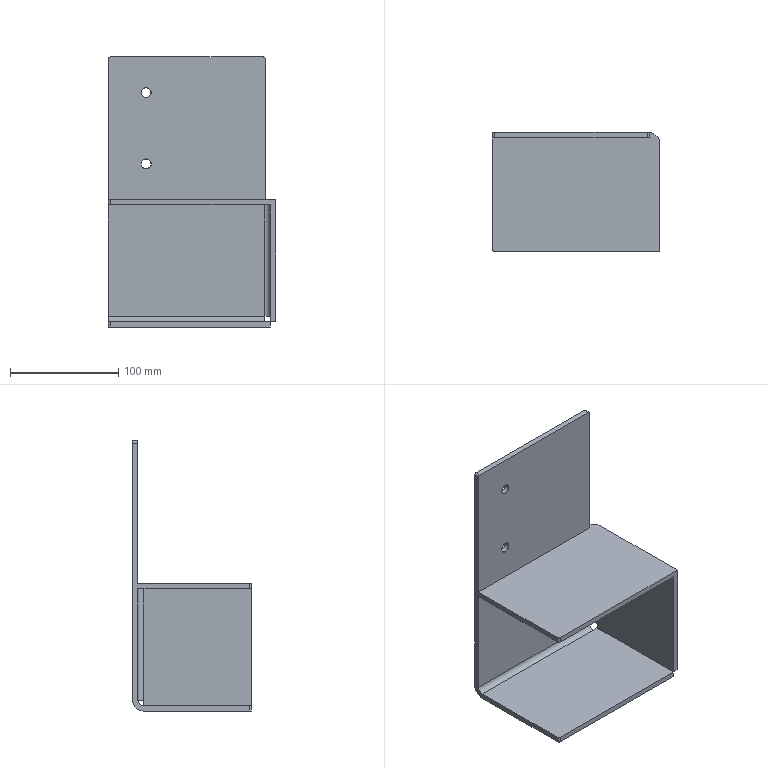Part | NX | 1 solid | 36 faces | box 155 x 110 x 250 mm | volume 398731 mm3 | plane 20 | cylinder 12 | cone 4 | commonest cylinder face diameters 4 x4 9 x4 10 x2 20 x2
STEP:
#1=CARTESIAN_POINT('',(44.,-222.5,-167.429));
#2=VERTEX_POINT('',#1);
#3=CARTESIAN_POINT('',(49.,-222.5,-167.429));
#4=VERTEX_POINT('',#3);
#5=CARTESIAN_POINT('',(49.,-222.5,-167.429));
#6=DIRECTION('',(1.,0.,0.));
#7=VECTOR('',#6,1000.);
#8=LINE('',#5,#7);
#9=EDGE_CURVE('',#2,#4,#8,.T.);
#10=ORIENTED_EDGE('',*,*,#9,.T.);
#11=CARTESIAN_POINT('',(49.,-322.5,-167.429));
#12=VERTEX_POINT('',#11);
#13=CARTESIAN_POINT('',(49.,-212.5,-167.429));
#14=DIRECTION('',(0.,-1.,0.));
#15=VECTOR('',#14,1000.);
#16=LINE('',#13,#15);
#17=EDGE_CURVE('',#4,#12,#16,.T.);
#18=ORIENTED_EDGE('',*,*,#17,.T.);
#19=CARTESIAN_POINT('',(44.,-322.5,-167.429));
#20=VERTEX_POINT('',#19);
#21=CARTESIAN_POINT('',(-35.923,-322.5,-167.429));
#22=DIRECTION('',(-1.,0.,0.));
#23=VECTOR('',#22,1000.);
#24=LINE('',#21,#23);
#25=EDGE_CURVE('',#12,#20,#24,.T.);
#26=ORIENTED_EDGE('',*,*,#25,.T.);
#27=CARTESIAN_POINT('',(44.,-212.5,-167.429));
#28=DIRECTION('',(0.,1.,0.));
#29=VECTOR('',#28,1000.);
#30=LINE('',#27,#29);
#31=EDGE_CURVE('',#20,#2,#30,.T.);
#32=ORIENTED_EDGE('',*,*,#31,.T.);
#33=EDGE_LOOP('',(#10,#18,#26,#32));
#34=FACE_BOUND('',#33,.T.);
#35=CARTESIAN_POINT('',(44.,-247.5,-167.429));
#36=DIRECTION('',(0.,0.,-1.));
#37=DIRECTION('',(0.,-1.,0.));
#38=AXIS2_PLACEMENT_3D('',#35,#36,#37);
#39=PLANE('',#38);
#40=ADVANCED_FACE('',(#34),#39,.T.);
#41=CARTESIAN_POINT('',(-106.,-320.5,-172.5));
#42=VERTEX_POINT('',#41);
#43=CARTESIAN_POINT('',(-106.,-320.5,-167.5));
#44=VERTEX_POINT('',#43);
#45=CARTESIAN_POINT('',(-106.,-320.5,-67.481));
#46=DIRECTION('',(0.,0.,1.));
#47=VECTOR('',#46,1000.);
#48=LINE('',#45,#47);
#49=EDGE_CURVE('',#42,#44,#48,.T.);
#50=ORIENTED_EDGE('',*,*,#49,.T.);
#51=CARTESIAN_POINT('',(-106.,-222.5,-167.5));
#52=VERTEX_POINT('',#51);
#53=CARTESIAN_POINT('',(-106.,-212.5,-167.5));
#54=DIRECTION('',(0.,1.,0.));
#55=VECTOR('',#54,1000.);
#56=LINE('',#53,#55);
#57=EDGE_CURVE('',#44,#52,#56,.T.);
#58=ORIENTED_EDGE('',*,*,#57,.T.);
#59=CARTESIAN_POINT('',(-106.,-217.5,-162.5));
#60=VERTEX_POINT('',#59);
#61=CARTESIAN_POINT('',(-106.,-222.5,-162.5));
#62=DIRECTION('',(1.,0.,0.));
#63=DIRECTION('',(0.,0.,-1.));
#64=AXIS2_PLACEMENT_3D('',#61,#62,#63);
#65=CIRCLE('',#64,5.);
#66=EDGE_CURVE('',#52,#60,#65,.T.);
#67=ORIENTED_EDGE('',*,*,#66,.T.);
#68=CARTESIAN_POINT('',(-106.,-217.5,-59.5));
#69=VERTEX_POINT('',#68);
#70=CARTESIAN_POINT('',(-106.,-217.5,-67.481));
#71=DIRECTION('',(0.,0.,1.));
#72=VECTOR('',#71,1000.);
#73=LINE('',#70,#72);
#74=EDGE_CURVE('',#60,#69,#73,.T.);
#75=ORIENTED_EDGE('',*,*,#74,.T.);
#76=CARTESIAN_POINT('',(-106.,-320.5,-59.5));
#77=VERTEX_POINT('',#76);
#78=CARTESIAN_POINT('',(-106.,-212.5,-59.5));
#79=DIRECTION('',(0.,-1.,0.));
#80=VECTOR('',#79,1000.);
#81=LINE('',#78,#80);
#82=EDGE_CURVE('',#69,#77,#81,.T.);
#83=ORIENTED_EDGE('',*,*,#82,.T.);
#84=CARTESIAN_POINT('',(-106.,-320.5,-54.5));
#85=VERTEX_POINT('',#84);
#86=CARTESIAN_POINT('',(-106.,-320.5,-67.481));
#87=DIRECTION('',(0.,0.,1.));
#88=VECTOR('',#87,1000.);
#89=LINE('',#86,#88);
#90=EDGE_CURVE('',#77,#85,#89,.T.);
#91=ORIENTED_EDGE('',*,*,#90,.T.);
#92=CARTESIAN_POINT('',(-106.,-217.5,-54.5));
#93=VERTEX_POINT('',#92);
#94=CARTESIAN_POINT('',(-106.,-212.5,-54.5));
#95=DIRECTION('',(0.,1.,0.));
#96=VECTOR('',#95,1000.);
#97=LINE('',#94,#96);
#98=EDGE_CURVE('',#85,#93,#97,.T.);
#99=ORIENTED_EDGE('',*,*,#98,.T.);
#100=CARTESIAN_POINT('',(-106.,-217.5,75.5));
#101=VERTEX_POINT('',#100);
#102=CARTESIAN_POINT('',(-106.,-217.5,-67.481));
#103=DIRECTION('',(0.,0.,1.));
#104=VECTOR('',#103,1000.);
#105=LINE('',#102,#104);
#106=EDGE_CURVE('',#93,#101,#105,.T.);
#107=ORIENTED_EDGE('',*,*,#106,.T.);
#108=CARTESIAN_POINT('',(-106.,-212.5,75.5));
#109=VERTEX_POINT('',#108);
#110=CARTESIAN_POINT('',(-106.,-212.5,75.5));
#111=DIRECTION('',(0.,-1.,0.));
#112=VECTOR('',#111,1000.);
#113=LINE('',#110,#112);
#114=EDGE_CURVE('',#109,#101,#113,.T.);
#115=ORIENTED_EDGE('',*,*,#114,.F.);
#116=CARTESIAN_POINT('',(-106.,-212.5,-162.5));
#117=VERTEX_POINT('',#116);
#118=CARTESIAN_POINT('',(-106.,-212.5,-67.481));
#119=DIRECTION('',(0.,0.,-1.));
#120=VECTOR('',#119,1000.);
#121=LINE('',#118,#120);
#122=EDGE_CURVE('',#109,#117,#121,.T.);
#123=ORIENTED_EDGE('',*,*,#122,.T.);
#124=CARTESIAN_POINT('',(-106.,-222.5,-172.5));
#125=VERTEX_POINT('',#124);
#126=CARTESIAN_POINT('',(-106.,-222.5,-162.5));
#127=DIRECTION('',(1.,0.,0.));
#128=DIRECTION('',(0.,0.,-1.));
#129=AXIS2_PLACEMENT_3D('',#126,#127,#128);
#130=CIRCLE('',#129,10.);
#131=EDGE_CURVE('',#125,#117,#130,.T.);
#132=ORIENTED_EDGE('',*,*,#131,.F.);
#133=CARTESIAN_POINT('',(-106.,-212.5,-172.5));
#134=DIRECTION('',(0.,-1.,0.));
#135=VECTOR('',#134,1000.);
#136=LINE('',#133,#135);
#137=EDGE_CURVE('',#125,#42,#136,.T.);
#138=ORIENTED_EDGE('',*,*,#137,.T.);
#139=EDGE_LOOP('',(#50,#58,#67,#75,#83,#91,#99,#107,#115,#123,#132,#138));
#140=FACE_BOUND('',#139,.T.);
#141=CARTESIAN_POINT('',(-106.,-212.5,-85.5));
#142=DIRECTION('',(-1.,0.,0.));
#143=DIRECTION('',(0.,0.,1.));
#144=AXIS2_PLACEMENT_3D('',#141,#142,#143);
#145=PLANE('',#144);
#146=ADVANCED_FACE('',(#140),#145,.T.);
#147=ORIENTED_EDGE('',*,*,#49,.F.);
#148=CARTESIAN_POINT('',(-104.,-322.5,-172.5));
#149=VERTEX_POINT('',#148);
#150=CARTESIAN_POINT('',(-104.,-320.5,-172.5));
#151=DIRECTION('',(0.,0.,1.));
#152=DIRECTION('',(1.,0.,0.));
#153=AXIS2_PLACEMENT_3D('',#150,#151,#152);
#154=CIRCLE('',#153,2.);
#155=EDGE_CURVE('',#42,#149,#154,.T.);
#156=ORIENTED_EDGE('',*,*,#155,.T.);
#157=CARTESIAN_POINT('',(-104.,-322.5,-167.5));
#158=VERTEX_POINT('',#157);
#159=CARTESIAN_POINT('',(-104.,-322.5,-67.481));
#160=DIRECTION('',(0.,0.,1.));
#161=VECTOR('',#160,1000.);
#162=LINE('',#159,#161);
#163=EDGE_CURVE('',#149,#158,#162,.T.);
#164=ORIENTED_EDGE('',*,*,#163,.T.);
#165=CARTESIAN_POINT('',(-104.,-320.5,-167.5));
#166=DIRECTION('',(0.,0.,1.));
#167=DIRECTION('',(1.,0.,0.));
#168=AXIS2_PLACEMENT_3D('',#165,#166,#167);
#169=CIRCLE('',#168,2.);
#170=EDGE_CURVE('',#44,#158,#169,.T.);
#171=ORIENTED_EDGE('',*,*,#170,.F.);
#172=EDGE_LOOP('',(#147,#156,#164,#171));
#173=FACE_BOUND('',#172,.T.);
#174=CARTESIAN_POINT('',(-104.,-320.5,-67.481));
#175=DIRECTION('',(0.,0.,1.));
#176=DIRECTION('',(1.,0.,0.));
#177=AXIS2_PLACEMENT_3D('',#174,#175,#176);
#178=CYLINDRICAL_SURFACE('',#177,2.);
#179=ADVANCED_FACE('',(#173),#178,.T.);
#180=CARTESIAN_POINT('',(37.5,-212.5,77.5));
#181=VERTEX_POINT('',#180);
#182=CARTESIAN_POINT('',(-104.,-212.5,77.5));
#183=VERTEX_POINT('',#182);
#184=CARTESIAN_POINT('',(-35.923,-212.5,77.5));
#185=DIRECTION('',(-1.,0.,0.));
#186=VECTOR('',#185,1000.);
#187=LINE('',#184,#186);
#188=EDGE_CURVE('',#181,#183,#187,.T.);
#189=ORIENTED_EDGE('',*,*,#188,.T.);
#190=CARTESIAN_POINT('',(-104.,-217.5,77.5));
#191=VERTEX_POINT('',#190);
#192=CARTESIAN_POINT('',(-104.,-212.5,77.5));
#193=DIRECTION('',(0.,-1.,0.));
#194=VECTOR('',#193,1000.);
#195=LINE('',#192,#194);
#196=EDGE_CURVE('',#183,#191,#195,.T.);
#197=ORIENTED_EDGE('',*,*,#196,.T.);
#198=CARTESIAN_POINT('',(37.5,-217.5,77.5));
#199=VERTEX_POINT('',#198);
#200=CARTESIAN_POINT('',(-35.923,-217.5,77.5));
#201=DIRECTION('',(1.,0.,0.));
#202=VECTOR('',#201,1000.);
#203=LINE('',#200,#202);
#204=EDGE_CURVE('',#191,#199,#203,.T.);
#205=ORIENTED_EDGE('',*,*,#204,.T.);
#206=CARTESIAN_POINT('',(37.5,-212.5,77.5));
#207=DIRECTION('',(0.,-1.,0.));
#208=VECTOR('',#207,1000.);
#209=LINE('',#206,#208);
#210=EDGE_CURVE('',#181,#199,#209,.T.);
#211=ORIENTED_EDGE('',*,*,#210,.F.);
#212=EDGE_LOOP('',(#189,#197,#205,#211));
#213=FACE_BOUND('',#212,.T.);
#214=CARTESIAN_POINT('',(49.,-122.093,77.5));
#215=DIRECTION('',(0.,0.,1.));
#216=DIRECTION('',(1.,0.,0.));
#217=AXIS2_PLACEMENT_3D('',#214,#215,#216);
#218=PLANE('',#217);
#219=ADVANCED_FACE('',(#213),#218,.T.);
#220=CARTESIAN_POINT('',(39.5,-212.513,75.5));
#221=VERTEX_POINT('',#220);
#222=CARTESIAN_POINT('',(39.5,-217.5,75.5));
#223=VERTEX_POINT('',#222);
#224=CARTESIAN_POINT('',(39.5,-212.5,75.5));
#225=DIRECTION('',(0.,-1.,0.));
#226=VECTOR('',#225,1000.);
#227=LINE('',#224,#226);
#228=EDGE_CURVE('',#221,#223,#227,.T.);
#229=ORIENTED_EDGE('',*,*,#228,.T.);
#230=CARTESIAN_POINT('',(39.5,-217.5,-54.5));
#231=VERTEX_POINT('',#230);
#232=CARTESIAN_POINT('',(39.5,-217.5,-67.481));
#233=DIRECTION('',(0.,0.,-1.));
#234=VECTOR('',#233,1000.);
#235=LINE('',#232,#234);
#236=EDGE_CURVE('',#223,#231,#235,.T.);
#237=ORIENTED_EDGE('',*,*,#236,.T.);
#238=CARTESIAN_POINT('',(39.5,-212.513,-54.5));
#239=VERTEX_POINT('',#238);
#240=CARTESIAN_POINT('',(39.5,-212.5,-54.5));
#241=DIRECTION('',(0.,-1.,0.));
#242=VECTOR('',#241,1000.);
#243=LINE('',#240,#242);
#244=EDGE_CURVE('',#239,#231,#243,.T.);
#245=ORIENTED_EDGE('',*,*,#244,.F.);
#246=CARTESIAN_POINT('',(39.5,-212.513,77.5));
#247=DIRECTION('',(0.,0.,1.));
#248=VECTOR('',#247,1000.);
#249=LINE('',#246,#248);
#250=EDGE_CURVE('',#239,#221,#249,.T.);
#251=ORIENTED_EDGE('',*,*,#250,.T.);
#252=EDGE_LOOP('',(#229,#237,#245,#251));
#253=FACE_BOUND('',#252,.T.);
#254=CARTESIAN_POINT('',(39.5,-201.5,-54.5));
#255=DIRECTION('',(-1.,0.,0.));
#256=DIRECTION('',(0.,0.,1.));
#257=AXIS2_PLACEMENT_3D('',#254,#255,#256);
#258=PLANE('',#257);
#259=ADVANCED_FACE('',(#253),#258,.F.);
#260=ORIENTED_EDGE('',*,*,#196,.F.);
#261=CARTESIAN_POINT('',(-104.,-212.5,75.5));
#262=DIRECTION('',(0.,-1.,0.));
#263=DIRECTION('',(1.,0.,0.));
#264=AXIS2_PLACEMENT_3D('',#261,#262,#263);
#265=CIRCLE('',#264,2.);
#266=EDGE_CURVE('',#183,#109,#265,.T.);
#267=ORIENTED_EDGE('',*,*,#266,.T.);
#268=ORIENTED_EDGE('',*,*,#114,.T.);
#269=CARTESIAN_POINT('',(-104.,-217.5,75.5));
#270=DIRECTION('',(0.,-1.,0.));
#271=DIRECTION('',(1.,0.,0.));
#272=AXIS2_PLACEMENT_3D('',#269,#270,#271);
#273=CIRCLE('',#272,2.);
#274=EDGE_CURVE('',#191,#101,#273,.T.);
#275=ORIENTED_EDGE('',*,*,#274,.F.);
#276=EDGE_LOOP('',(#260,#267,#268,#275));
#277=FACE_BOUND('',#276,.T.);
#278=CARTESIAN_POINT('',(-104.,-212.5,75.5));
#279=DIRECTION('',(0.,-1.,0.));
#280=DIRECTION('',(1.,0.,0.));
#281=AXIS2_PLACEMENT_3D('',#278,#279,#280);
#282=CYLINDRICAL_SURFACE('',#281,2.);
#283=ADVANCED_FACE('',(#277),#282,.T.);
#284=ORIENTED_EDGE('',*,*,#228,.F.);
#285=CARTESIAN_POINT('',(39.,-212.5,76.823));
#286=VERTEX_POINT('',#285);
#287=CARTESIAN_POINT('',(39.5,-212.513,75.5));
#288=CARTESIAN_POINT('',(39.5,-212.513,75.53));
#289=CARTESIAN_POINT('',(39.5,-212.512,75.56));
#290=CARTESIAN_POINT('',(39.498,-212.512,75.591));
#291=CARTESIAN_POINT('',(39.497,-212.512,75.621));
#292=CARTESIAN_POINT('',(39.495,-212.512,75.651));
#293=CARTESIAN_POINT('',(39.492,-212.512,75.681));
#294=CARTESIAN_POINT('',(39.489,-212.512,75.711));
#295=CARTESIAN_POINT('',(39.486,-212.512,75.741));
#296=CARTESIAN_POINT('',(39.482,-212.512,75.77));
#297=CARTESIAN_POINT('',(39.478,-212.511,75.8));
#298=CARTESIAN_POINT('',(39.473,-212.511,75.83));
#299=CARTESIAN_POINT('',(39.468,-212.511,75.859));
#300=CARTESIAN_POINT('',(39.462,-212.511,75.889));
#301=CARTESIAN_POINT('',(39.456,-212.51,75.918));
#302=CARTESIAN_POINT('',(39.45,-212.51,75.947));
#303=CARTESIAN_POINT('',(39.443,-212.51,75.977));
#304=CARTESIAN_POINT('',(39.435,-212.509,76.006));
#305=CARTESIAN_POINT('',(39.427,-212.509,76.035));
#306=CARTESIAN_POINT('',(39.419,-212.509,76.064));
#307=CARTESIAN_POINT('',(39.411,-212.508,76.093));
#308=CARTESIAN_POINT('',(39.401,-212.508,76.122));
#309=CARTESIAN_POINT('',(39.392,-212.508,76.15));
#310=CARTESIAN_POINT('',(39.382,-212.507,76.179));
#311=CARTESIAN_POINT('',(39.371,-212.507,76.207));
#312=CARTESIAN_POINT('',(39.36,-212.506,76.236));
#313=CARTESIAN_POINT('',(39.349,-212.506,76.264));
#314=CARTESIAN_POINT('',(39.337,-212.506,76.291));
#315=CARTESIAN_POINT('',(39.325,-212.505,76.319));
#316=CARTESIAN_POINT('',(39.313,-212.505,76.347));
#317=CARTESIAN_POINT('',(39.299,-212.504,76.374));
#318=CARTESIAN_POINT('',(39.286,-212.504,76.401));
#319=CARTESIAN_POINT('',(39.272,-212.504,76.428));
#320=CARTESIAN_POINT('',(39.258,-212.503,76.454));
#321=CARTESIAN_POINT('',(39.244,-212.503,76.48));
#322=CARTESIAN_POINT('',(39.229,-212.503,76.506));
#323=CARTESIAN_POINT('',(39.213,-212.502,76.532));
#324=CARTESIAN_POINT('',(39.182,-212.502,76.583));
#325=CARTESIAN_POINT('',(39.149,-212.501,76.633));
#326=CARTESIAN_POINT('',(39.114,-212.501,76.682));
#327=CARTESIAN_POINT('',(39.096,-212.5,76.706));
#328=CARTESIAN_POINT('',(39.077,-212.5,76.73));
#329=CARTESIAN_POINT('',(39.058,-212.5,76.754));
#330=CARTESIAN_POINT('',(39.039,-212.5,76.777));
#331=CARTESIAN_POINT('',(39.02,-212.5,76.8));
#332=CARTESIAN_POINT('',(39.,-212.5,76.823));
#333=B_SPLINE_CURVE_WITH_KNOTS('',3,(#287,#288,#289,#290,#291,#292,#293,#294,#295,#296,#297,#298,#299,#300,#301,#302,#303,#304,#305,#306,#307,#308,#309,#310,#311,#312,#313,#314,#315,#316,#317,#318,#319,#320,#321,#322,#323,#324,#325,#326,#327,#328,#329,#330,#331,#332),.UNSPECIFIED.,.F.,.F.,(4,3,3,3,3,3,3,3,3,3,3,3,3,3,3,4),(0.,0.09059,0.181,0.2711,0.361,0.4512,0.5417,0.6323,0.723,0.8136,0.9042,0.9945,1.085,1.265,1.355,1.446),.UNSPECIFIED.);
#334=EDGE_CURVE('',#221,#286,#333,.T.);
#335=ORIENTED_EDGE('',*,*,#334,.T.);
#336=CARTESIAN_POINT('',(37.5,-212.5,75.5));
#337=DIRECTION('',(0.,-1.,0.));
#338=DIRECTION('',(1.,0.,0.));
#339=AXIS2_PLACEMENT_3D('',#336,#337,#338);
#340=CIRCLE('',#339,2.);
#341=EDGE_CURVE('',#286,#181,#340,.T.);
#342=ORIENTED_EDGE('',*,*,#341,.T.);
#343=ORIENTED_EDGE('',*,*,#210,.T.);
#344=CARTESIAN_POINT('',(37.5,-217.5,75.5));
#345=DIRECTION('',(0.,-1.,0.));
#346=DIRECTION('',(1.,0.,0.));
#347=AXIS2_PLACEMENT_3D('',#344,#345,#346);
#348=CIRCLE('',#347,2.);
#349=EDGE_CURVE('',#223,#199,#348,.T.);
#350=ORIENTED_EDGE('',*,*,#349,.F.);
#351=EDGE_LOOP('',(#284,#335,#342,#343,#350));
#352=FACE_BOUND('',#351,.T.);
#353=CARTESIAN_POINT('',(37.5,-212.5,75.5));
#354=DIRECTION('',(0.,-1.,0.));
#355=DIRECTION('',(1.,0.,0.));
#356=AXIS2_PLACEMENT_3D('',#353,#354,#355);
#357=CYLINDRICAL_SURFACE('',#356,2.);
#358=ADVANCED_FACE('',(#352),#357,.T.);
#359=ORIENTED_EDGE('',*,*,#31,.F.);
#360=CARTESIAN_POINT('',(44.,-322.5,-59.5));
#361=VERTEX_POINT('',#360);
#362=CARTESIAN_POINT('',(44.,-322.5,-67.481));
#363=DIRECTION('',(0.,0.,-1.));
#364=VECTOR('',#363,1000.);
#365=LINE('',#362,#364);
#366=EDGE_CURVE('',#361,#20,#365,.T.);
#367=ORIENTED_EDGE('',*,*,#366,.F.);
#368=CARTESIAN_POINT('',(44.,-222.5,-59.5));
#369=VERTEX_POINT('',#368);
#370=CARTESIAN_POINT('',(44.,-212.5,-59.5));
#371=DIRECTION('',(0.,1.,0.));
#372=VECTOR('',#371,1000.);
#373=LINE('',#370,#372);
#374=EDGE_CURVE('',#361,#369,#373,.T.);
#375=ORIENTED_EDGE('',*,*,#374,.T.);
#376=CARTESIAN_POINT('',(44.,-222.5,-162.5));
#377=VERTEX_POINT('',#376);
#378=CARTESIAN_POINT('',(44.,-222.5,-67.481));
#379=DIRECTION('',(0.,0.,1.));
#380=VECTOR('',#379,1000.);
#381=LINE('',#378,#380);
#382=EDGE_CURVE('',#377,#369,#381,.T.);
#383=ORIENTED_EDGE('',*,*,#382,.F.);
#384=CARTESIAN_POINT('',(44.,-222.5,-67.481));
#385=DIRECTION('',(0.,0.,1.));
#386=VECTOR('',#385,1000.);
#387=LINE('',#384,#386);
#388=EDGE_CURVE('',#2,#377,#387,.T.);
#389=ORIENTED_EDGE('',*,*,#388,.F.);
#390=EDGE_LOOP('',(#359,#367,#375,#383,#389));
#391=FACE_BOUND('',#390,.T.);
#392=CARTESIAN_POINT('',(44.,-222.093,-172.5));
#393=DIRECTION('',(1.,0.,0.));
#394=DIRECTION('',(0.,1.,0.));
#395=AXIS2_PLACEMENT_3D('',#392,#393,#394);
#396=PLANE('',#395);
#397=ADVANCED_FACE('',(#391),#396,.F.);
#398=CARTESIAN_POINT('',(-104.,-322.5,-59.5));
#399=VERTEX_POINT('',#398);
#400=CARTESIAN_POINT('',(-104.,-322.5,-54.5));
#401=VERTEX_POINT('',#400);
#402=CARTESIAN_POINT('',(-104.,-322.5,-67.481));
#403=DIRECTION('',(0.,0.,1.));
#404=VECTOR('',#403,1000.);
#405=LINE('',#402,#404);
#406=EDGE_CURVE('',#399,#401,#405,.T.);
#407=ORIENTED_EDGE('',*,*,#406,.F.);
#408=CARTESIAN_POINT('',(-35.923,-322.5,-59.5));
#409=DIRECTION('',(-1.,0.,0.));
#410=VECTOR('',#409,1000.);
#411=LINE('',#408,#410);
#412=EDGE_CURVE('',#361,#399,#411,.T.);
#413=ORIENTED_EDGE('',*,*,#412,.F.);
#414=ORIENTED_EDGE('',*,*,#366,.T.);
#415=ORIENTED_EDGE('',*,*,#25,.F.);
#416=CARTESIAN_POINT('',(49.,-322.5,-54.5));
#417=VERTEX_POINT('',#416);
#418=CARTESIAN_POINT('',(49.,-322.5,-67.481));
#419=DIRECTION('',(0.,0.,1.));
#420=VECTOR('',#419,1000.);
#421=LINE('',#418,#420);
#422=EDGE_CURVE('',#12,#417,#421,.T.);
#423=ORIENTED_EDGE('',*,*,#422,.T.);
#424=CARTESIAN_POINT('',(-35.923,-322.5,-54.5));
#425=DIRECTION('',(1.,0.,0.));
#426=VECTOR('',#425,1000.);
#427=LINE('',#424,#426);
#428=EDGE_CURVE('',#401,#417,#427,.T.);
#429=ORIENTED_EDGE('',*,*,#428,.F.);
#430=EDGE_LOOP('',(#407,#413,#414,#415,#423,#429));
#431=FACE_BOUND('',#430,.T.);
#432=CARTESIAN_POINT('',(-27.527,-322.5,-83.375));
#433=DIRECTION('',(0.,-1.,0.));
#434=DIRECTION('',(0.,0.,-1.));
#435=AXIS2_PLACEMENT_3D('',#432,#433,#434);
#436=PLANE('',#435);
#437=ADVANCED_FACE('',(#431),#436,.T.);
#438=ORIENTED_EDGE('',*,*,#428,.T.);
#439=CARTESIAN_POINT('',(49.,-222.5,-54.5));
#440=VERTEX_POINT('',#439);
#441=CARTESIAN_POINT('',(49.,-212.5,-54.5));
#442=DIRECTION('',(0.,-1.,0.));
#443=VECTOR('',#442,1000.);
#444=LINE('',#441,#443);
#445=EDGE_CURVE('',#440,#417,#444,.T.);
#446=ORIENTED_EDGE('',*,*,#445,.F.);
#447=CARTESIAN_POINT('',(39.,-222.5,-54.5));
#448=DIRECTION('',(0.,0.,1.));
#449=DIRECTION('',(1.,0.,0.));
#450=AXIS2_PLACEMENT_3D('',#447,#448,#449);
#451=CIRCLE('',#450,10.);
#452=EDGE_CURVE('',#440,#239,#451,.T.);
#453=ORIENTED_EDGE('',*,*,#452,.T.);
#454=ORIENTED_EDGE('',*,*,#244,.T.);
#455=CARTESIAN_POINT('',(-35.923,-217.5,-54.5));
#456=DIRECTION('',(1.,0.,0.));
#457=VECTOR('',#456,1000.);
#458=LINE('',#455,#457);
#459=EDGE_CURVE('',#93,#231,#458,.T.);
#460=ORIENTED_EDGE('',*,*,#459,.F.);
#461=ORIENTED_EDGE('',*,*,#98,.F.);
#462=CARTESIAN_POINT('',(-104.,-320.5,-54.5));
#463=DIRECTION('',(0.,0.,1.));
#464=DIRECTION('',(1.,0.,0.));
#465=AXIS2_PLACEMENT_3D('',#462,#463,#464);
#466=CIRCLE('',#465,2.);
#467=EDGE_CURVE('',#85,#401,#466,.T.);
#468=ORIENTED_EDGE('',*,*,#467,.T.);
#469=EDGE_LOOP('',(#438,#446,#453,#454,#460,#461,#468));
#470=FACE_BOUND('',#469,.T.);
#471=CARTESIAN_POINT('',(-106.,-217.5,-54.5));
#472=DIRECTION('',(0.,0.,1.));
#473=DIRECTION('',(1.,0.,0.));
#474=AXIS2_PLACEMENT_3D('',#471,#472,#473);
#475=PLANE('',#474);
#476=ADVANCED_FACE('',(#470),#475,.T.);
#477=CARTESIAN_POINT('',(-75.5,-217.3,-21.5));
#478=VERTEX_POINT('',#477);
#479=CARTESIAN_POINT('',(-66.5,-217.3,-21.5));
#480=VERTEX_POINT('',#479);
#481=CARTESIAN_POINT('',(-71.,-217.3,-21.5));
#482=DIRECTION('',(0.,-1.,0.));
#483=DIRECTION('',(1.,0.,0.));
#484=AXIS2_PLACEMENT_3D('',#481,#482,#483);
#485=CIRCLE('',#484,4.5);
#486=EDGE_CURVE('',#478,#480,#485,.T.);
#487=ORIENTED_EDGE('',*,*,#486,.T.);
#488=CARTESIAN_POINT('',(-66.5,-212.5,-21.5));
#489=VERTEX_POINT('',#488);
#490=CARTESIAN_POINT('',(-66.5,-217.5,-21.5));
#491=DIRECTION('',(0.,-1.,0.));
#492=VECTOR('',#491,1000.);
#493=LINE('',#490,#492);
#494=EDGE_CURVE('',#489,#480,#493,.T.);
#495=ORIENTED_EDGE('',*,*,#494,.F.);
#496=CARTESIAN_POINT('',(-75.5,-212.5,-21.5));
#497=VERTEX_POINT('',#496);
#498=CARTESIAN_POINT('',(-71.,-212.5,-21.5));
#499=DIRECTION('',(0.,-1.,0.));
#500=DIRECTION('',(1.,0.,0.));
#501=AXIS2_PLACEMENT_3D('',#498,#499,#500);
#502=CIRCLE('',#501,4.5);
#503=EDGE_CURVE('',#497,#489,#502,.T.);
#504=ORIENTED_EDGE('',*,*,#503,.F.);
#505=CARTESIAN_POINT('',(-75.5,-217.5,-21.5));
#506=DIRECTION('',(0.,-1.,0.));
#507=VECTOR('',#506,1000.);
#508=LINE('',#505,#507);
#509=EDGE_CURVE('',#497,#478,#508,.T.);
#510=ORIENTED_EDGE('',*,*,#509,.T.);
#511=EDGE_LOOP('',(#487,#495,#504,#510));
#512=FACE_BOUND('',#511,.T.);
#513=CARTESIAN_POINT('',(-71.,-217.5,-21.5));
#514=DIRECTION('',(0.,-1.,0.));
#515=DIRECTION('',(1.,0.,0.));
#516=AXIS2_PLACEMENT_3D('',#513,#514,#515);
#517=CYLINDRICAL_SURFACE('',#516,4.5);
#518=ADVANCED_FACE('',(#512),#517,.F.);
#519=CARTESIAN_POINT('',(49.,-222.5,-162.5));
#520=VERTEX_POINT('',#519);
#521=CARTESIAN_POINT('',(49.,-222.5,-67.481));
#522=DIRECTION('',(0.,0.,1.));
#523=VECTOR('',#522,1000.);
#524=LINE('',#521,#523);
#525=EDGE_CURVE('',#4,#520,#524,.T.);
#526=ORIENTED_EDGE('',*,*,#525,.F.);
#527=ORIENTED_EDGE('',*,*,#9,.F.);
#528=ORIENTED_EDGE('',*,*,#388,.T.);
#529=CARTESIAN_POINT('',(49.,-222.5,-162.5));
#530=DIRECTION('',(-1.,0.,0.));
#531=VECTOR('',#530,1000.);
#532=LINE('',#529,#531);
#533=EDGE_CURVE('',#520,#377,#532,.T.);
#534=ORIENTED_EDGE('',*,*,#533,.F.);
#535=EDGE_LOOP('',(#526,#527,#528,#534));
#536=FACE_BOUND('',#535,.T.);
#537=CARTESIAN_POINT('',(49.,-222.5,-172.907));
#538=DIRECTION('',(0.,1.,0.));
#539=DIRECTION('',(1.,0.,0.));
#540=AXIS2_PLACEMENT_3D('',#537,#538,#539);
#541=PLANE('',#540);
#542=ADVANCED_FACE('',(#536),#541,.T.);
#543=CARTESIAN_POINT('',(39.,-212.5,-162.5));
#544=VERTEX_POINT('',#543);
#545=CARTESIAN_POINT('',(39.,-222.5,-162.5));
#546=DIRECTION('',(0.,0.,1.));
#547=DIRECTION('',(1.,0.,0.));
#548=AXIS2_PLACEMENT_3D('',#545,#546,#547);
#549=CIRCLE('',#548,10.);
#550=EDGE_CURVE('',#520,#544,#549,.T.);
#551=ORIENTED_EDGE('',*,*,#550,.F.);
#552=ORIENTED_EDGE('',*,*,#533,.T.);
#553=CARTESIAN_POINT('',(39.,-217.5,-162.5));
#554=VERTEX_POINT('',#553);
#555=CARTESIAN_POINT('',(39.,-222.5,-162.5));
#556=DIRECTION('',(0.,0.,-1.));
#557=DIRECTION('',(0.,1.,0.));
#558=AXIS2_PLACEMENT_3D('',#555,#556,#557);
#559=CIRCLE('',#558,5.);
#560=EDGE_CURVE('',#554,#377,#559,.T.);
#561=ORIENTED_EDGE('',*,*,#560,.F.);
#562=CARTESIAN_POINT('',(39.,-212.5,-162.5));
#563=DIRECTION('',(0.,-1.,0.));
#564=VECTOR('',#563,1000.);
#565=LINE('',#562,#564);
#566=EDGE_CURVE('',#544,#554,#565,.T.);
#567=ORIENTED_EDGE('',*,*,#566,.F.);
#568=EDGE_LOOP('',(#551,#552,#561,#567));
#569=FACE_BOUND('',#568,.T.);
#570=CARTESIAN_POINT('',(39.,-222.5,-162.5));
#571=DIRECTION('',(0.,0.,1.));
#572=DIRECTION('',(1.,0.,0.));
#573=AXIS2_PLACEMENT_3D('',#570,#571,#572);
#574=PLANE('',#573);
#575=ADVANCED_FACE('',(#569),#574,.F.);
#576=CARTESIAN_POINT('',(-35.923,-217.5,-162.5));
#577=DIRECTION('',(1.,0.,0.));
#578=VECTOR('',#577,1000.);
#579=LINE('',#576,#578);
#580=EDGE_CURVE('',#60,#554,#579,.T.);
#581=ORIENTED_EDGE('',*,*,#580,.F.);
#582=ORIENTED_EDGE('',*,*,#66,.F.);
#583=CARTESIAN_POINT('',(39.,-222.5,-167.5));
#584=VERTEX_POINT('',#583);
#585=CARTESIAN_POINT('',(-35.923,-222.5,-167.5));
#586=DIRECTION('',(1.,0.,0.));
#587=VECTOR('',#586,1000.);
#588=LINE('',#585,#587);
#589=EDGE_CURVE('',#52,#584,#588,.T.);
#590=ORIENTED_EDGE('',*,*,#589,.T.);
#591=CARTESIAN_POINT('',(39.,-222.5,-162.5));
#592=DIRECTION('',(-1.,0.,0.));
#593=DIRECTION('',(0.,1.,0.));
#594=AXIS2_PLACEMENT_3D('',#591,#592,#593);
#595=CIRCLE('',#594,5.);
#596=EDGE_CURVE('',#554,#584,#595,.T.);
#597=ORIENTED_EDGE('',*,*,#596,.F.);
#598=EDGE_LOOP('',(#581,#582,#590,#597));
#599=FACE_BOUND('',#598,.T.);
#600=CARTESIAN_POINT('',(39.,-222.5,-162.5));
#601=DIRECTION('',(1.,0.,0.));
#602=DIRECTION('',(0.,0.,-1.));
#603=AXIS2_PLACEMENT_3D('',#600,#601,#602);
#604=CYLINDRICAL_SURFACE('',#603,5.);
#605=ADVANCED_FACE('',(#599),#604,.F.);
#606=ORIENTED_EDGE('',*,*,#589,.F.);
#607=ORIENTED_EDGE('',*,*,#57,.F.);
#608=ORIENTED_EDGE('',*,*,#170,.T.);
#609=CARTESIAN_POINT('',(43.929,-322.5,-167.5));
#610=VERTEX_POINT('',#609);
#611=CARTESIAN_POINT('',(-35.923,-322.5,-167.5));
#612=DIRECTION('',(-1.,0.,0.));
#613=VECTOR('',#612,1000.);
#614=LINE('',#611,#613);
#615=EDGE_CURVE('',#610,#158,#614,.T.);
#616=ORIENTED_EDGE('',*,*,#615,.F.);
#617=CARTESIAN_POINT('',(43.929,-222.5,-167.5));
#618=VERTEX_POINT('',#617);
#619=CARTESIAN_POINT('',(43.929,-212.5,-167.5));
#620=DIRECTION('',(0.,1.,0.));
#621=VECTOR('',#620,1000.);
#622=LINE('',#619,#621);
#623=EDGE_CURVE('',#610,#618,#622,.T.);
#624=ORIENTED_EDGE('',*,*,#623,.T.);
#625=CARTESIAN_POINT('',(-35.923,-222.5,-167.5));
#626=DIRECTION('',(1.,0.,0.));
#627=VECTOR('',#626,1000.);
#628=LINE('',#625,#627);
#629=EDGE_CURVE('',#584,#618,#628,.T.);
#630=ORIENTED_EDGE('',*,*,#629,.F.);
#631=EDGE_LOOP('',(#606,#607,#608,#616,#624,#630));
#632=FACE_BOUND('',#631,.T.);
#633=CARTESIAN_POINT('',(49.,-222.093,-167.5));
#634=DIRECTION('',(0.,0.,-1.));
#635=DIRECTION('',(0.,-1.,0.));
#636=AXIS2_PLACEMENT_3D('',#633,#634,#635);
#637=PLANE('',#636);
#638=ADVANCED_FACE('',(#632),#637,.F.);
#639=CARTESIAN_POINT('',(39.,-217.5,-59.5));
#640=VERTEX_POINT('',#639);
#641=CARTESIAN_POINT('',(39.,-222.5,-59.5));
#642=DIRECTION('',(0.,0.,1.));
#643=DIRECTION('',(1.,0.,0.));
#644=AXIS2_PLACEMENT_3D('',#641,#642,#643);
#645=CIRCLE('',#644,5.);
#646=EDGE_CURVE('',#369,#640,#645,.T.);
#647=ORIENTED_EDGE('',*,*,#646,.T.);
#648=CARTESIAN_POINT('',(39.,-217.5,-67.481));
#649=DIRECTION('',(0.,0.,1.));
#650=VECTOR('',#649,1000.);
#651=LINE('',#648,#650);
#652=EDGE_CURVE('',#554,#640,#651,.T.);
#653=ORIENTED_EDGE('',*,*,#652,.F.);
#654=ORIENTED_EDGE('',*,*,#560,.T.);
#655=ORIENTED_EDGE('',*,*,#382,.T.);
#656=EDGE_LOOP('',(#647,#653,#654,#655));
#657=FACE_BOUND('',#656,.T.);
#658=CARTESIAN_POINT('',(39.,-222.5,77.5));
#659=DIRECTION('',(0.,0.,1.));
#660=DIRECTION('',(1.,0.,0.));
#661=AXIS2_PLACEMENT_3D('',#658,#659,#660);
#662=CYLINDRICAL_SURFACE('',#661,5.);
#663=ADVANCED_FACE('',(#657),#662,.F.);
#664=CARTESIAN_POINT('',(-35.923,-217.5,-59.5));
#665=DIRECTION('',(-1.,0.,0.));
#666=VECTOR('',#665,1000.);
#667=LINE('',#664,#666);
#668=EDGE_CURVE('',#640,#69,#667,.T.);
#669=ORIENTED_EDGE('',*,*,#668,.T.);
#670=ORIENTED_EDGE('',*,*,#74,.F.);
#671=ORIENTED_EDGE('',*,*,#580,.T.);
#672=ORIENTED_EDGE('',*,*,#652,.T.);
#673=EDGE_LOOP('',(#669,#670,#671,#672));
#674=FACE_BOUND('',#673,.T.);
#675=CARTESIAN_POINT('',(49.,-217.5,-172.5));
#676=DIRECTION('',(0.,1.,0.));
#677=DIRECTION('',(1.,0.,0.));
#678=AXIS2_PLACEMENT_3D('',#675,#676,#677);
#679=PLANE('',#678);
#680=ADVANCED_FACE('',(#674),#679,.F.);
#681=ORIENTED_EDGE('',*,*,#486,.F.);
#682=CARTESIAN_POINT('',(-75.7,-217.5,-21.5));
#683=VERTEX_POINT('',#682);
#684=CARTESIAN_POINT('',(-75.5,-217.3,-21.5));
#685=DIRECTION('',(-0.7071,-0.7071,0.));
#686=VECTOR('',#685,1000.);
#687=LINE('',#684,#686);
#688=EDGE_CURVE('',#478,#683,#687,.T.);
#689=ORIENTED_EDGE('',*,*,#688,.T.);
#690=CARTESIAN_POINT('',(-66.3,-217.5,-21.5));
#691=VERTEX_POINT('',#690);
#692=CARTESIAN_POINT('',(-71.,-217.5,-21.5));
#693=DIRECTION('',(0.,-1.,0.));
#694=DIRECTION('',(1.,0.,0.));
#695=AXIS2_PLACEMENT_3D('',#692,#693,#694);
#696=CIRCLE('',#695,4.7);
#697=EDGE_CURVE('',#683,#691,#696,.T.);
#698=ORIENTED_EDGE('',*,*,#697,.T.);
#699=CARTESIAN_POINT('',(-66.5,-217.3,-21.5));
#700=DIRECTION('',(0.7071,-0.7071,0.));
#701=VECTOR('',#700,1000.);
#702=LINE('',#699,#701);
#703=EDGE_CURVE('',#480,#691,#702,.T.);
#704=ORIENTED_EDGE('',*,*,#703,.F.);
#705=EDGE_LOOP('',(#681,#689,#698,#704));
#706=FACE_BOUND('',#705,.T.);
#707=CARTESIAN_POINT('',(-71.,-217.3,-21.5));
#708=DIRECTION('',(0.,-1.,0.));
#709=DIRECTION('',(1.,0.,0.));
#710=AXIS2_PLACEMENT_3D('',#707,#708,#709);
#711=CONICAL_SURFACE('',#710,4.5,0.7854);
#712=ADVANCED_FACE('',(#706),#711,.F.);
#713=ORIENTED_EDGE('',*,*,#236,.F.);
#714=ORIENTED_EDGE('',*,*,#349,.T.);
#715=ORIENTED_EDGE('',*,*,#204,.F.);
#716=ORIENTED_EDGE('',*,*,#274,.T.);
#717=ORIENTED_EDGE('',*,*,#106,.F.);
#718=ORIENTED_EDGE('',*,*,#459,.T.);
#719=EDGE_LOOP('',(#713,#714,#715,#716,#717,#718));
#720=FACE_BOUND('',#719,.T.);
#721=ORIENTED_EDGE('',*,*,#697,.F.);
#722=CARTESIAN_POINT('',(-71.,-217.5,-21.5));
#723=DIRECTION('',(0.,-1.,0.));
#724=DIRECTION('',(1.,0.,0.));
#725=AXIS2_PLACEMENT_3D('',#722,#723,#724);
#726=CIRCLE('',#725,4.7);
#727=EDGE_CURVE('',#691,#683,#726,.T.);
#728=ORIENTED_EDGE('',*,*,#727,.F.);
#729=EDGE_LOOP('',(#721,#728));
#730=FACE_BOUND('',#729,.T.);
#731=CARTESIAN_POINT('',(-75.7,-217.5,44.5));
#732=VERTEX_POINT('',#731);
#733=CARTESIAN_POINT('',(-66.3,-217.5,44.5));
#734=VERTEX_POINT('',#733);
#735=CARTESIAN_POINT('',(-71.,-217.5,44.5));
#736=DIRECTION('',(0.,-1.,0.));
#737=DIRECTION('',(1.,0.,0.));
#738=AXIS2_PLACEMENT_3D('',#735,#736,#737);
#739=CIRCLE('',#738,4.7);
#740=EDGE_CURVE('',#732,#734,#739,.T.);
#741=ORIENTED_EDGE('',*,*,#740,.F.);
#742=CARTESIAN_POINT('',(-71.,-217.5,44.5));
#743=DIRECTION('',(0.,-1.,0.));
#744=DIRECTION('',(1.,0.,0.));
#745=AXIS2_PLACEMENT_3D('',#742,#743,#744);
#746=CIRCLE('',#745,4.7);
#747=EDGE_CURVE('',#734,#732,#746,.T.);
#748=ORIENTED_EDGE('',*,*,#747,.F.);
#749=EDGE_LOOP('',(#741,#748));
#750=FACE_BOUND('',#749,.T.);
#751=CARTESIAN_POINT('',(46.157,-217.5,34.808));
#752=DIRECTION('',(0.,-1.,0.));
#753=DIRECTION('',(0.,0.,-1.));
#754=AXIS2_PLACEMENT_3D('',#751,#752,#753);
#755=PLANE('',#754);
#756=ADVANCED_FACE('',(#720,#730,#750),#755,.T.);
#757=ORIENTED_EDGE('',*,*,#668,.F.);
#758=ORIENTED_EDGE('',*,*,#646,.F.);
#759=ORIENTED_EDGE('',*,*,#374,.F.);
#760=ORIENTED_EDGE('',*,*,#412,.T.);
#761=CARTESIAN_POINT('',(-104.,-320.5,-59.5));
#762=DIRECTION('',(0.,0.,1.));
#763=DIRECTION('',(1.,0.,0.));
#764=AXIS2_PLACEMENT_3D('',#761,#762,#763);
#765=CIRCLE('',#764,2.);
#766=EDGE_CURVE('',#77,#399,#765,.T.);
#767=ORIENTED_EDGE('',*,*,#766,.F.);
#768=ORIENTED_EDGE('',*,*,#82,.F.);
#769=EDGE_LOOP('',(#757,#758,#759,#760,#767,#768));
#770=FACE_BOUND('',#769,.T.);
#771=CARTESIAN_POINT('',(44.,-217.5,-59.5));
#772=DIRECTION('',(0.,0.,-1.));
#773=DIRECTION('',(0.,-1.,0.));
#774=AXIS2_PLACEMENT_3D('',#771,#772,#773);
#775=PLANE('',#774);
#776=ADVANCED_FACE('',(#770),#775,.T.);
#777=ORIENTED_EDGE('',*,*,#406,.T.);
#778=ORIENTED_EDGE('',*,*,#467,.F.);
#779=ORIENTED_EDGE('',*,*,#90,.F.);
#780=ORIENTED_EDGE('',*,*,#766,.T.);
#781=EDGE_LOOP('',(#777,#778,#779,#780));
#782=FACE_BOUND('',#781,.T.);
#783=CARTESIAN_POINT('',(-104.,-320.5,-67.481));
#784=DIRECTION('',(0.,0.,1.));
#785=DIRECTION('',(1.,0.,0.));
#786=AXIS2_PLACEMENT_3D('',#783,#784,#785);
#787=CYLINDRICAL_SURFACE('',#786,2.);
#788=ADVANCED_FACE('',(#782),#787,.T.);
#789=CARTESIAN_POINT('',(-75.5,-217.3,44.5));
#790=VERTEX_POINT('',#789);
#791=CARTESIAN_POINT('',(-66.5,-217.3,44.5));
#792=VERTEX_POINT('',#791);
#793=CARTESIAN_POINT('',(-71.,-217.3,44.5));
#794=DIRECTION('',(0.,-1.,0.));
#795=DIRECTION('',(1.,0.,0.));
#796=AXIS2_PLACEMENT_3D('',#793,#794,#795);
#797=CIRCLE('',#796,4.5);
#798=EDGE_CURVE('',#790,#792,#797,.T.);
#799=ORIENTED_EDGE('',*,*,#798,.T.);
#800=CARTESIAN_POINT('',(-66.5,-212.5,44.5));
#801=VERTEX_POINT('',#800);
#802=CARTESIAN_POINT('',(-66.5,-217.5,44.5));
#803=DIRECTION('',(0.,-1.,0.));
#804=VECTOR('',#803,1000.);
#805=LINE('',#802,#804);
#806=EDGE_CURVE('',#801,#792,#805,.T.);
#807=ORIENTED_EDGE('',*,*,#806,.F.);
#808=CARTESIAN_POINT('',(-75.5,-212.5,44.5));
#809=VERTEX_POINT('',#808);
#810=CARTESIAN_POINT('',(-71.,-212.5,44.5));
#811=DIRECTION('',(0.,-1.,0.));
#812=DIRECTION('',(1.,0.,0.));
#813=AXIS2_PLACEMENT_3D('',#810,#811,#812);
#814=CIRCLE('',#813,4.5);
#815=EDGE_CURVE('',#809,#801,#814,.T.);
#816=ORIENTED_EDGE('',*,*,#815,.F.);
#817=CARTESIAN_POINT('',(-75.5,-217.5,44.5));
#818=DIRECTION('',(0.,-1.,0.));
#819=VECTOR('',#818,1000.);
#820=LINE('',#817,#819);
#821=EDGE_CURVE('',#809,#790,#820,.T.);
#822=ORIENTED_EDGE('',*,*,#821,.T.);
#823=EDGE_LOOP('',(#799,#807,#816,#822));
#824=FACE_BOUND('',#823,.T.);
#825=CARTESIAN_POINT('',(-71.,-217.5,44.5));
#826=DIRECTION('',(0.,-1.,0.));
#827=DIRECTION('',(1.,0.,0.));
#828=AXIS2_PLACEMENT_3D('',#825,#826,#827);
#829=CYLINDRICAL_SURFACE('',#828,4.5);
#830=ADVANCED_FACE('',(#824),#829,.F.);
#831=ORIENTED_EDGE('',*,*,#798,.F.);
#832=CARTESIAN_POINT('',(-75.5,-217.3,44.5));
#833=DIRECTION('',(-0.7071,-0.7071,0.));
#834=VECTOR('',#833,1000.);
#835=LINE('',#832,#834);
#836=EDGE_CURVE('',#790,#732,#835,.T.);
#837=ORIENTED_EDGE('',*,*,#836,.T.);
#838=ORIENTED_EDGE('',*,*,#740,.T.);
#839=CARTESIAN_POINT('',(-66.5,-217.3,44.5));
#840=DIRECTION('',(0.7071,-0.7071,0.));
#841=VECTOR('',#840,1000.);
#842=LINE('',#839,#841);
#843=EDGE_CURVE('',#792,#734,#842,.T.);
#844=ORIENTED_EDGE('',*,*,#843,.F.);
#845=EDGE_LOOP('',(#831,#837,#838,#844));
#846=FACE_BOUND('',#845,.T.);
#847=CARTESIAN_POINT('',(-71.,-217.3,44.5));
#848=DIRECTION('',(0.,-1.,0.));
#849=DIRECTION('',(1.,0.,0.));
#850=AXIS2_PLACEMENT_3D('',#847,#848,#849);
#851=CONICAL_SURFACE('',#850,4.5,0.7854);
#852=ADVANCED_FACE('',(#846),#851,.F.);
#853=ORIENTED_EDGE('',*,*,#494,.T.);
#854=CARTESIAN_POINT('',(-71.,-217.3,-21.5));
#855=DIRECTION('',(0.,-1.,0.));
#856=DIRECTION('',(1.,0.,0.));
#857=AXIS2_PLACEMENT_3D('',#854,#855,#856);
#858=CIRCLE('',#857,4.5);
#859=EDGE_CURVE('',#480,#478,#858,.T.);
#860=ORIENTED_EDGE('',*,*,#859,.T.);
#861=ORIENTED_EDGE('',*,*,#509,.F.);
#862=CARTESIAN_POINT('',(-71.,-212.5,-21.5));
#863=DIRECTION('',(0.,-1.,0.));
#864=DIRECTION('',(1.,0.,0.));
#865=AXIS2_PLACEMENT_3D('',#862,#863,#864);
#866=CIRCLE('',#865,4.5);
#867=EDGE_CURVE('',#489,#497,#866,.T.);
#868=ORIENTED_EDGE('',*,*,#867,.F.);
#869=EDGE_LOOP('',(#853,#860,#861,#868));
#870=FACE_BOUND('',#869,.T.);
#871=CARTESIAN_POINT('',(-71.,-217.5,-21.5));
#872=DIRECTION('',(0.,-1.,0.));
#873=DIRECTION('',(1.,0.,0.));
#874=AXIS2_PLACEMENT_3D('',#871,#872,#873);
#875=CYLINDRICAL_SURFACE('',#874,4.5);
#876=ADVANCED_FACE('',(#870),#875,.F.);
#877=ORIENTED_EDGE('',*,*,#806,.T.);
#878=CARTESIAN_POINT('',(-71.,-217.3,44.5));
#879=DIRECTION('',(0.,-1.,0.));
#880=DIRECTION('',(1.,0.,0.));
#881=AXIS2_PLACEMENT_3D('',#878,#879,#880);
#882=CIRCLE('',#881,4.5);
#883=EDGE_CURVE('',#792,#790,#882,.T.);
#884=ORIENTED_EDGE('',*,*,#883,.T.);
#885=ORIENTED_EDGE('',*,*,#821,.F.);
#886=CARTESIAN_POINT('',(-71.,-212.5,44.5));
#887=DIRECTION('',(0.,-1.,0.));
#888=DIRECTION('',(1.,0.,0.));
#889=AXIS2_PLACEMENT_3D('',#886,#887,#888);
#890=CIRCLE('',#889,4.5);
#891=EDGE_CURVE('',#801,#809,#890,.T.);
#892=ORIENTED_EDGE('',*,*,#891,.F.);
#893=EDGE_LOOP('',(#877,#884,#885,#892));
#894=FACE_BOUND('',#893,.T.);
#895=CARTESIAN_POINT('',(-71.,-217.5,44.5));
#896=DIRECTION('',(0.,-1.,0.));
#897=DIRECTION('',(1.,0.,0.));
#898=AXIS2_PLACEMENT_3D('',#895,#896,#897);
#899=CYLINDRICAL_SURFACE('',#898,4.5);
#900=ADVANCED_FACE('',(#894),#899,.F.);
#901=ORIENTED_EDGE('',*,*,#703,.T.);
#902=ORIENTED_EDGE('',*,*,#727,.T.);
#903=ORIENTED_EDGE('',*,*,#688,.F.);
#904=ORIENTED_EDGE('',*,*,#859,.F.);
#905=EDGE_LOOP('',(#901,#902,#903,#904));
#906=FACE_BOUND('',#905,.T.);
#907=CARTESIAN_POINT('',(-71.,-217.3,-21.5));
#908=DIRECTION('',(0.,-1.,0.));
#909=DIRECTION('',(1.,0.,0.));
#910=AXIS2_PLACEMENT_3D('',#907,#908,#909);
#911=CONICAL_SURFACE('',#910,4.5,0.7854);
#912=ADVANCED_FACE('',(#906),#911,.F.);
#913=ORIENTED_EDGE('',*,*,#843,.T.);
#914=ORIENTED_EDGE('',*,*,#747,.T.);
#915=ORIENTED_EDGE('',*,*,#836,.F.);
#916=ORIENTED_EDGE('',*,*,#883,.F.);
#917=EDGE_LOOP('',(#913,#914,#915,#916));
#918=FACE_BOUND('',#917,.T.);
#919=CARTESIAN_POINT('',(-71.,-217.3,44.5));
#920=DIRECTION('',(0.,-1.,0.));
#921=DIRECTION('',(1.,0.,0.));
#922=AXIS2_PLACEMENT_3D('',#919,#920,#921);
#923=CONICAL_SURFACE('',#922,4.5,0.7854);
#924=ADVANCED_FACE('',(#918),#923,.F.);
#925=CARTESIAN_POINT('',(39.,-222.5,-172.5));
#926=VERTEX_POINT('',#925);
#927=CARTESIAN_POINT('',(39.,-222.5,-162.5));
#928=DIRECTION('',(1.,0.,0.));
#929=DIRECTION('',(0.,0.,-1.));
#930=AXIS2_PLACEMENT_3D('',#927,#928,#929);
#931=CIRCLE('',#930,10.);
#932=EDGE_CURVE('',#926,#544,#931,.T.);
#933=ORIENTED_EDGE('',*,*,#932,.T.);
#934=ORIENTED_EDGE('',*,*,#566,.T.);
#935=ORIENTED_EDGE('',*,*,#596,.T.);
#936=CARTESIAN_POINT('',(39.,-222.5,-172.5));
#937=DIRECTION('',(0.,0.,1.));
#938=VECTOR('',#937,1000.);
#939=LINE('',#936,#938);
#940=EDGE_CURVE('',#926,#584,#939,.T.);
#941=ORIENTED_EDGE('',*,*,#940,.F.);
#942=EDGE_LOOP('',(#933,#934,#935,#941));
#943=FACE_BOUND('',#942,.T.);
#944=CARTESIAN_POINT('',(39.,-222.5,-162.5));
#945=DIRECTION('',(1.,0.,0.));
#946=DIRECTION('',(0.,0.,1.));
#947=AXIS2_PLACEMENT_3D('',#944,#945,#946);
#948=PLANE('',#947);
#949=ADVANCED_FACE('',(#943),#948,.T.);
#950=CARTESIAN_POINT('',(43.929,-222.5,-172.5));
#951=VERTEX_POINT('',#950);
#952=CARTESIAN_POINT('',(43.929,-222.5,-172.5));
#953=DIRECTION('',(0.,0.,1.));
#954=VECTOR('',#953,1000.);
#955=LINE('',#952,#954);
#956=EDGE_CURVE('',#951,#618,#955,.T.);
#957=ORIENTED_EDGE('',*,*,#956,.T.);
#958=ORIENTED_EDGE('',*,*,#623,.F.);
#959=CARTESIAN_POINT('',(43.929,-322.5,-172.5));
#960=VERTEX_POINT('',#959);
#961=CARTESIAN_POINT('',(43.929,-322.5,-67.481));
#962=DIRECTION('',(0.,0.,-1.));
#963=VECTOR('',#962,1000.);
#964=LINE('',#961,#963);
#965=EDGE_CURVE('',#610,#960,#964,.T.);
#966=ORIENTED_EDGE('',*,*,#965,.T.);
#967=CARTESIAN_POINT('',(43.929,-212.5,-172.5));
#968=DIRECTION('',(0.,1.,0.));
#969=VECTOR('',#968,1000.);
#970=LINE('',#967,#969);
#971=EDGE_CURVE('',#960,#951,#970,.T.);
#972=ORIENTED_EDGE('',*,*,#971,.T.);
#973=EDGE_LOOP('',(#957,#958,#966,#972));
#974=FACE_BOUND('',#973,.T.);
#975=CARTESIAN_POINT('',(43.929,-222.093,-172.5));
#976=DIRECTION('',(1.,0.,0.));
#977=DIRECTION('',(0.,0.,1.));
#978=AXIS2_PLACEMENT_3D('',#975,#976,#977);
#979=PLANE('',#978);
#980=ADVANCED_FACE('',(#974),#979,.T.);
#981=ORIENTED_EDGE('',*,*,#956,.F.);
#982=CARTESIAN_POINT('',(-35.923,-222.5,-172.5));
#983=DIRECTION('',(-1.,0.,0.));
#984=VECTOR('',#983,1000.);
#985=LINE('',#982,#984);
#986=EDGE_CURVE('',#951,#926,#985,.T.);
#987=ORIENTED_EDGE('',*,*,#986,.T.);
#988=ORIENTED_EDGE('',*,*,#940,.T.);
#989=ORIENTED_EDGE('',*,*,#629,.T.);
#990=EDGE_LOOP('',(#981,#987,#988,#989));
#991=FACE_BOUND('',#990,.T.);
#992=CARTESIAN_POINT('',(39.,-222.5,-172.5));
#993=DIRECTION('',(0.,1.,0.));
#994=DIRECTION('',(1.,0.,0.));
#995=AXIS2_PLACEMENT_3D('',#992,#993,#994);
#996=PLANE('',#995);
#997=ADVANCED_FACE('',(#991),#996,.T.);
#998=CARTESIAN_POINT('',(-35.923,-322.5,-172.5));
#999=DIRECTION('',(1.,0.,0.));
#1000=VECTOR('',#999,1000.);
#1001=LINE('',#998,#1000);
#1002=EDGE_CURVE('',#149,#960,#1001,.T.);
#1003=ORIENTED_EDGE('',*,*,#1002,.T.);
#1004=ORIENTED_EDGE('',*,*,#965,.F.);
#1005=ORIENTED_EDGE('',*,*,#615,.T.);
#1006=ORIENTED_EDGE('',*,*,#163,.F.);
#1007=EDGE_LOOP('',(#1003,#1004,#1005,#1006));
#1008=FACE_BOUND('',#1007,.T.);
#1009=CARTESIAN_POINT('',(43.929,-322.5,-172.5));
#1010=DIRECTION('',(0.,-1.,0.));
#1011=DIRECTION('',(0.,0.,-1.));
#1012=AXIS2_PLACEMENT_3D('',#1009,#1010,#1011);
#1013=PLANE('',#1012);
#1014=ADVANCED_FACE('',(#1008),#1013,.T.);
#1015=CARTESIAN_POINT('',(39.,-212.5,-67.481));
#1016=DIRECTION('',(0.,0.,-1.));
#1017=VECTOR('',#1016,1000.);
#1018=LINE('',#1015,#1017);
#1019=EDGE_CURVE('',#286,#544,#1018,.T.);
#1020=ORIENTED_EDGE('',*,*,#1019,.T.);
#1021=CARTESIAN_POINT('',(-35.923,-212.5,-162.5));
#1022=DIRECTION('',(-1.,0.,0.));
#1023=VECTOR('',#1022,1000.);
#1024=LINE('',#1021,#1023);
#1025=EDGE_CURVE('',#544,#117,#1024,.T.);
#1026=ORIENTED_EDGE('',*,*,#1025,.T.);
#1027=ORIENTED_EDGE('',*,*,#122,.F.);
#1028=ORIENTED_EDGE('',*,*,#266,.F.);
#1029=ORIENTED_EDGE('',*,*,#188,.F.);
#1030=ORIENTED_EDGE('',*,*,#341,.F.);
#1031=EDGE_LOOP('',(#1020,#1026,#1027,#1028,#1029,#1030));
#1032=FACE_BOUND('',#1031,.T.);
#1033=ORIENTED_EDGE('',*,*,#503,.T.);
#1034=ORIENTED_EDGE('',*,*,#867,.T.);
#1035=EDGE_LOOP('',(#1033,#1034));
#1036=FACE_BOUND('',#1035,.T.);
#1037=ORIENTED_EDGE('',*,*,#815,.T.);
#1038=ORIENTED_EDGE('',*,*,#891,.T.);
#1039=EDGE_LOOP('',(#1037,#1038));
#1040=FACE_BOUND('',#1039,.T.);
#1041=CARTESIAN_POINT('',(-35.923,-212.5,-67.481));
#1042=DIRECTION('',(0.,-1.,0.));
#1043=DIRECTION('',(0.,0.,-1.));
#1044=AXIS2_PLACEMENT_3D('',#1041,#1042,#1043);
#1045=PLANE('',#1044);
#1046=ADVANCED_FACE('',(#1032,#1036,#1040),#1045,.F.);
#1047=ORIENTED_EDGE('',*,*,#1019,.F.);
#1048=ORIENTED_EDGE('',*,*,#334,.F.);
#1049=ORIENTED_EDGE('',*,*,#250,.F.);
#1050=ORIENTED_EDGE('',*,*,#452,.F.);
#1051=CARTESIAN_POINT('',(49.,-222.5,-67.481));
#1052=DIRECTION('',(0.,0.,-1.));
#1053=VECTOR('',#1052,1000.);
#1054=LINE('',#1051,#1053);
#1055=EDGE_CURVE('',#440,#520,#1054,.T.);
#1056=ORIENTED_EDGE('',*,*,#1055,.T.);
#1057=ORIENTED_EDGE('',*,*,#550,.T.);
#1058=EDGE_LOOP('',(#1047,#1048,#1049,#1050,#1056,#1057));
#1059=FACE_BOUND('',#1058,.T.);
#1060=CARTESIAN_POINT('',(39.,-222.5,77.5));
#1061=DIRECTION('',(0.,0.,1.));
#1062=DIRECTION('',(1.,0.,0.));
#1063=AXIS2_PLACEMENT_3D('',#1060,#1061,#1062);
#1064=CYLINDRICAL_SURFACE('',#1063,10.);
#1065=ADVANCED_FACE('',(#1059),#1064,.T.);
#1066=ORIENTED_EDGE('',*,*,#525,.T.);
#1067=ORIENTED_EDGE('',*,*,#1055,.F.);
#1068=ORIENTED_EDGE('',*,*,#445,.T.);
#1069=ORIENTED_EDGE('',*,*,#422,.F.);
#1070=ORIENTED_EDGE('',*,*,#17,.F.);
#1071=EDGE_LOOP('',(#1066,#1067,#1068,#1069,#1070));
#1072=FACE_BOUND('',#1071,.T.);
#1073=CARTESIAN_POINT('',(49.,-137.171,-67.481));
#1074=DIRECTION('',(-1.,0.,0.));
#1075=DIRECTION('',(0.,0.,1.));
#1076=AXIS2_PLACEMENT_3D('',#1073,#1074,#1075);
#1077=PLANE('',#1076);
#1078=ADVANCED_FACE('',(#1072),#1077,.F.);
#1079=ORIENTED_EDGE('',*,*,#1025,.F.);
#1080=ORIENTED_EDGE('',*,*,#932,.F.);
#1081=CARTESIAN_POINT('',(-35.923,-222.5,-172.5));
#1082=DIRECTION('',(-1.,0.,0.));
#1083=VECTOR('',#1082,1000.);
#1084=LINE('',#1081,#1083);
#1085=EDGE_CURVE('',#926,#125,#1084,.T.);
#1086=ORIENTED_EDGE('',*,*,#1085,.T.);
#1087=ORIENTED_EDGE('',*,*,#131,.T.);
#1088=EDGE_LOOP('',(#1079,#1080,#1086,#1087));
#1089=FACE_BOUND('',#1088,.T.);
#1090=CARTESIAN_POINT('',(39.,-222.5,-162.5));
#1091=DIRECTION('',(1.,0.,0.));
#1092=DIRECTION('',(0.,0.,-1.));
#1093=AXIS2_PLACEMENT_3D('',#1090,#1091,#1092);
#1094=CYLINDRICAL_SURFACE('',#1093,10.);
#1095=ADVANCED_FACE('',(#1089),#1094,.T.);
#1096=ORIENTED_EDGE('',*,*,#1085,.F.);
#1097=ORIENTED_EDGE('',*,*,#986,.F.);
#1098=ORIENTED_EDGE('',*,*,#971,.F.);
#1099=ORIENTED_EDGE('',*,*,#1002,.F.);
#1100=ORIENTED_EDGE('',*,*,#155,.F.);
#1101=ORIENTED_EDGE('',*,*,#137,.F.);
#1102=EDGE_LOOP('',(#1096,#1097,#1098,#1099,#1100,#1101));
#1103=FACE_BOUND('',#1102,.T.);
#1104=CARTESIAN_POINT('',(-35.923,-117.074,-172.5));
#1105=DIRECTION('',(0.,0.,1.));
#1106=DIRECTION('',(1.,0.,0.));
#1107=AXIS2_PLACEMENT_3D('',#1104,#1105,#1106);
#1108=PLANE('',#1107);
#1109=ADVANCED_FACE('',(#1103),#1108,.F.);
#1110=CLOSED_SHELL('',(#40,#146,#179,#219,#259,#283,#358,#397,#437,#476,#518,#542,#575,#605,#638,#663,#680,#712,#756,#776,#788,#830,#852,#876,#900,#912,#924,#949,#980,#997,#1014,#1046,#1065,#1078,#1095,#1109));
#1111=MANIFOLD_SOLID_BREP('',#1110);
#1112=(LENGTH_UNIT()NAMED_UNIT(*)SI_UNIT(.MILLI.,.METRE.));
#1113=UNCERTAINTY_MEASURE_WITH_UNIT(LENGTH_MEASURE(0.00001),#1112,'','');
#1114=(NAMED_UNIT(*)PLANE_ANGLE_UNIT()SI_UNIT($,.RADIAN.));
#1115=(NAMED_UNIT(*)SI_UNIT($,.STERADIAN.)SOLID_ANGLE_UNIT());
#1116=(GEOMETRIC_REPRESENTATION_CONTEXT(3)GLOBAL_UNCERTAINTY_ASSIGNED_CONTEXT((#1113))GLOBAL_UNIT_ASSIGNED_CONTEXT((#1112,#1114,#1115))REPRESENTATION_CONTEXT('',''));
#1117=ADVANCED_BREP_SHAPE_REPRESENTATION('',(#1111),#1116);